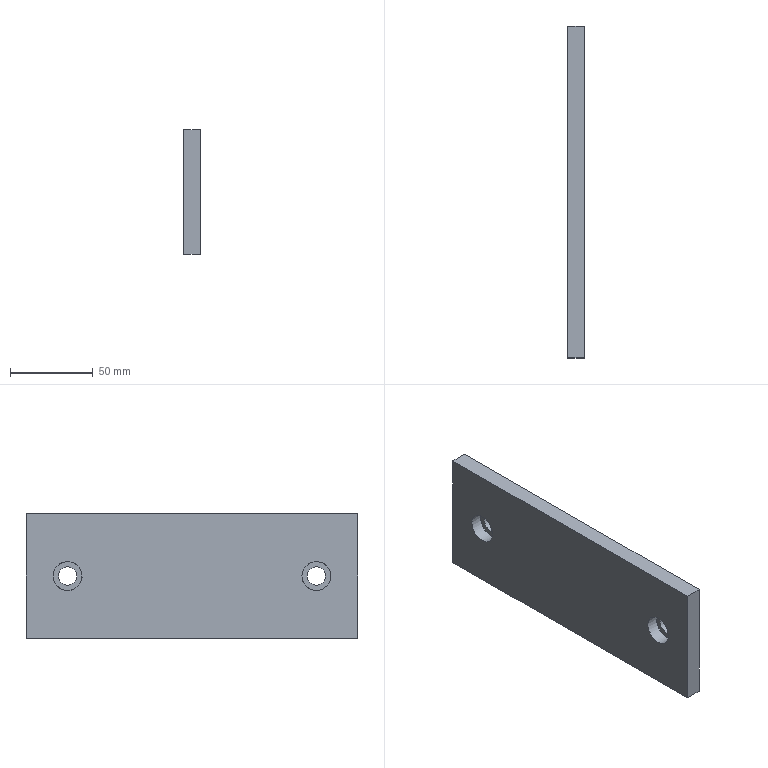Part | NX | features solid 2 | 1 solid | 12 faces | box 10 x 200 x 75 mm | volume 145975 mm3 | plane 8 | cylinder 4 | commonest cylinder face diameters 11 x2 17.5 x2
STEP:
#1=CARTESIAN_POINT('',(-680.,-535.,290.));
#2=VERTEX_POINT('',#1);
#3=CARTESIAN_POINT('',(-680.,-535.,215.));
#4=VERTEX_POINT('',#3);
#5=CARTESIAN_POINT('',(-680.,-535.,210.));
#6=DIRECTION('',(0.,0.,-1.));
#7=VECTOR('',#6,1000.);
#8=LINE('',#5,#7);
#9=EDGE_CURVE('',#2,#4,#8,.T.);
#10=ORIENTED_EDGE('',*,*,#9,.T.);
#11=CARTESIAN_POINT('',(-670.,-535.,215.));
#12=VERTEX_POINT('',#11);
#13=CARTESIAN_POINT('',(-670.,-535.,215.));
#14=DIRECTION('',(-1.,0.,0.));
#15=VECTOR('',#14,1000.);
#16=LINE('',#13,#15);
#17=EDGE_CURVE('',#12,#4,#16,.T.);
#18=ORIENTED_EDGE('',*,*,#17,.F.);
#19=CARTESIAN_POINT('',(-670.,-535.,290.));
#20=VERTEX_POINT('',#19);
#21=CARTESIAN_POINT('',(-670.,-535.,210.));
#22=DIRECTION('',(0.,0.,1.));
#23=VECTOR('',#22,1000.);
#24=LINE('',#21,#23);
#25=EDGE_CURVE('',#20,#12,#24,.F.);
#26=ORIENTED_EDGE('',*,*,#25,.F.);
#27=CARTESIAN_POINT('',(-670.,-535.,290.));
#28=DIRECTION('',(-1.,0.,0.));
#29=VECTOR('',#28,1000.);
#30=LINE('',#27,#29);
#31=EDGE_CURVE('',#20,#2,#30,.T.);
#32=ORIENTED_EDGE('',*,*,#31,.T.);
#33=EDGE_LOOP('',(#10,#18,#26,#32));
#34=FACE_BOUND('',#33,.T.);
#35=CARTESIAN_POINT('',(-670.,-535.,210.));
#36=DIRECTION('',(0.,1.,0.));
#37=DIRECTION('',(-1.,0.,0.));
#38=AXIS2_PLACEMENT_3D('',#35,#36,#37);
#39=PLANE('',#38);
#40=ADVANCED_FACE('',(#34),#39,.F.);
#41=CARTESIAN_POINT('',(-680.,-335.,290.));
#42=VERTEX_POINT('',#41);
#43=CARTESIAN_POINT('',(-680.,-485.,290.));
#44=DIRECTION('',(0.,-1.,0.));
#45=VECTOR('',#44,1000.);
#46=LINE('',#43,#45);
#47=EDGE_CURVE('',#42,#2,#46,.T.);
#48=ORIENTED_EDGE('',*,*,#47,.T.);
#49=ORIENTED_EDGE('',*,*,#31,.F.);
#50=CARTESIAN_POINT('',(-670.,-335.,290.));
#51=VERTEX_POINT('',#50);
#52=CARTESIAN_POINT('',(-670.,-485.,290.));
#53=DIRECTION('',(0.,-1.,0.));
#54=VECTOR('',#53,1000.);
#55=LINE('',#52,#54);
#56=EDGE_CURVE('',#51,#20,#55,.T.);
#57=ORIENTED_EDGE('',*,*,#56,.F.);
#58=CARTESIAN_POINT('',(-670.,-335.,290.));
#59=DIRECTION('',(-1.,0.,0.));
#60=VECTOR('',#59,1000.);
#61=LINE('',#58,#60);
#62=EDGE_CURVE('',#51,#42,#61,.T.);
#63=ORIENTED_EDGE('',*,*,#62,.T.);
#64=EDGE_LOOP('',(#48,#49,#57,#63));
#65=FACE_BOUND('',#64,.T.);
#66=CARTESIAN_POINT('',(-670.,-485.,290.));
#67=DIRECTION('',(0.,0.,-1.));
#68=DIRECTION('',(1.,0.,0.));
#69=AXIS2_PLACEMENT_3D('',#66,#67,#68);
#70=PLANE('',#69);
#71=ADVANCED_FACE('',(#65),#70,.F.);
#72=CARTESIAN_POINT('',(-680.,-335.,215.));
#73=VERTEX_POINT('',#72);
#74=CARTESIAN_POINT('',(-680.,-335.,268.));
#75=DIRECTION('',(0.,0.,1.));
#76=VECTOR('',#75,1000.);
#77=LINE('',#74,#76);
#78=EDGE_CURVE('',#73,#42,#77,.T.);
#79=ORIENTED_EDGE('',*,*,#78,.T.);
#80=ORIENTED_EDGE('',*,*,#62,.F.);
#81=CARTESIAN_POINT('',(-670.,-335.,215.));
#82=VERTEX_POINT('',#81);
#83=CARTESIAN_POINT('',(-670.,-335.,268.));
#84=DIRECTION('',(0.,0.,-1.));
#85=VECTOR('',#84,1000.);
#86=LINE('',#83,#85);
#87=EDGE_CURVE('',#82,#51,#86,.F.);
#88=ORIENTED_EDGE('',*,*,#87,.F.);
#89=CARTESIAN_POINT('',(-670.,-335.,215.));
#90=DIRECTION('',(-1.,0.,0.));
#91=VECTOR('',#90,1000.);
#92=LINE('',#89,#91);
#93=EDGE_CURVE('',#82,#73,#92,.T.);
#94=ORIENTED_EDGE('',*,*,#93,.T.);
#95=EDGE_LOOP('',(#79,#80,#88,#94));
#96=FACE_BOUND('',#95,.T.);
#97=CARTESIAN_POINT('',(-670.,-335.,268.));
#98=DIRECTION('',(0.,-1.,0.));
#99=DIRECTION('',(1.,0.,0.));
#100=AXIS2_PLACEMENT_3D('',#97,#98,#99);
#101=PLANE('',#100);
#102=ADVANCED_FACE('',(#96),#101,.F.);
#103=CARTESIAN_POINT('',(-680.,-335.,215.));
#104=DIRECTION('',(0.,1.,0.));
#105=VECTOR('',#104,1000.);
#106=LINE('',#103,#105);
#107=EDGE_CURVE('',#4,#73,#106,.T.);
#108=ORIENTED_EDGE('',*,*,#107,.T.);
#109=ORIENTED_EDGE('',*,*,#93,.F.);
#110=CARTESIAN_POINT('',(-670.,-485.,215.));
#111=DIRECTION('',(0.,1.,0.));
#112=VECTOR('',#111,1000.);
#113=LINE('',#110,#112);
#114=EDGE_CURVE('',#12,#82,#113,.T.);
#115=ORIENTED_EDGE('',*,*,#114,.F.);
#116=ORIENTED_EDGE('',*,*,#17,.T.);
#117=EDGE_LOOP('',(#108,#109,#115,#116));
#118=FACE_BOUND('',#117,.T.);
#119=CARTESIAN_POINT('',(-670.,-335.,215.));
#120=DIRECTION('',(0.,0.,1.));
#121=DIRECTION('',(0.,1.,0.));
#122=AXIS2_PLACEMENT_3D('',#119,#120,#121);
#123=PLANE('',#122);
#124=ADVANCED_FACE('',(#118),#123,.F.);
#125=CARTESIAN_POINT('',(-672.7,-501.25,252.5));
#126=VERTEX_POINT('',#125);
#127=CARTESIAN_POINT('',(-672.7,-510.,252.5));
#128=DIRECTION('',(-1.,0.,0.));
#129=DIRECTION('',(0.,1.,0.));
#130=AXIS2_PLACEMENT_3D('',#127,#128,#129);
#131=CIRCLE('',#130,8.75);
#132=EDGE_CURVE('',#126,#126,#131,.T.);
#133=ORIENTED_EDGE('',*,*,#132,.F.);
#134=EDGE_LOOP('',(#133));
#135=FACE_BOUND('',#134,.T.);
#136=CARTESIAN_POINT('',(-680.,-510.,243.75));
#137=VERTEX_POINT('',#136);
#138=CARTESIAN_POINT('',(-680.,-510.,252.5));
#139=DIRECTION('',(1.,0.,0.));
#140=DIRECTION('',(0.,0.,-1.));
#141=AXIS2_PLACEMENT_3D('',#138,#139,#140);
#142=CIRCLE('',#141,8.75);
#143=EDGE_CURVE('',#137,#137,#142,.F.);
#144=ORIENTED_EDGE('',*,*,#143,.T.);
#145=EDGE_LOOP('',(#144));
#146=FACE_BOUND('',#145,.T.);
#147=CARTESIAN_POINT('',(-690.,-510.,252.5));
#148=DIRECTION('',(1.,0.,0.));
#149=DIRECTION('',(0.,1.,0.));
#150=AXIS2_PLACEMENT_3D('',#147,#148,#149);
#151=CYLINDRICAL_SURFACE('',#150,8.75);
#152=ADVANCED_FACE('',(#135,#146),#151,.F.);
#153=CARTESIAN_POINT('',(-672.7,-351.25,252.5));
#154=VERTEX_POINT('',#153);
#155=CARTESIAN_POINT('',(-672.7,-360.,252.5));
#156=DIRECTION('',(-1.,0.,0.));
#157=DIRECTION('',(0.,1.,0.));
#158=AXIS2_PLACEMENT_3D('',#155,#156,#157);
#159=CIRCLE('',#158,8.75);
#160=EDGE_CURVE('',#154,#154,#159,.T.);
#161=ORIENTED_EDGE('',*,*,#160,.F.);
#162=EDGE_LOOP('',(#161));
#163=FACE_BOUND('',#162,.T.);
#164=CARTESIAN_POINT('',(-680.,-360.,243.75));
#165=VERTEX_POINT('',#164);
#166=CARTESIAN_POINT('',(-680.,-360.,252.5));
#167=DIRECTION('',(1.,0.,0.));
#168=DIRECTION('',(0.,0.,-1.));
#169=AXIS2_PLACEMENT_3D('',#166,#167,#168);
#170=CIRCLE('',#169,8.75);
#171=EDGE_CURVE('',#165,#165,#170,.F.);
#172=ORIENTED_EDGE('',*,*,#171,.T.);
#173=EDGE_LOOP('',(#172));
#174=FACE_BOUND('',#173,.T.);
#175=CARTESIAN_POINT('',(-690.,-360.,252.5));
#176=DIRECTION('',(1.,0.,0.));
#177=DIRECTION('',(0.,1.,0.));
#178=AXIS2_PLACEMENT_3D('',#175,#176,#177);
#179=CYLINDRICAL_SURFACE('',#178,8.75);
#180=ADVANCED_FACE('',(#163,#174),#179,.F.);
#181=CARTESIAN_POINT('',(-670.,-354.5,252.5));
#182=VERTEX_POINT('',#181);
#183=CARTESIAN_POINT('',(-670.,-360.,252.5));
#184=DIRECTION('',(-1.,0.,0.));
#185=DIRECTION('',(0.,1.,0.));
#186=AXIS2_PLACEMENT_3D('',#183,#184,#185);
#187=CIRCLE('',#186,5.5);
#188=EDGE_CURVE('',#182,#182,#187,.T.);
#189=ORIENTED_EDGE('',*,*,#188,.T.);
#190=EDGE_LOOP('',(#189));
#191=FACE_BOUND('',#190,.T.);
#192=CARTESIAN_POINT('',(-670.,-504.5,252.5));
#193=VERTEX_POINT('',#192);
#194=CARTESIAN_POINT('',(-670.,-510.,252.5));
#195=DIRECTION('',(-1.,0.,0.));
#196=DIRECTION('',(0.,1.,0.));
#197=AXIS2_PLACEMENT_3D('',#194,#195,#196);
#198=CIRCLE('',#197,5.5);
#199=EDGE_CURVE('',#193,#193,#198,.T.);
#200=ORIENTED_EDGE('',*,*,#199,.T.);
#201=EDGE_LOOP('',(#200));
#202=FACE_BOUND('',#201,.T.);
#203=ORIENTED_EDGE('',*,*,#87,.T.);
#204=ORIENTED_EDGE('',*,*,#56,.T.);
#205=ORIENTED_EDGE('',*,*,#25,.T.);
#206=ORIENTED_EDGE('',*,*,#114,.T.);
#207=EDGE_LOOP('',(#203,#204,#205,#206));
#208=FACE_BOUND('',#207,.T.);
#209=CARTESIAN_POINT('',(-670.,-485.,268.));
#210=DIRECTION('',(1.,0.,0.));
#211=DIRECTION('',(0.,1.,0.));
#212=AXIS2_PLACEMENT_3D('',#209,#210,#211);
#213=PLANE('',#212);
#214=ADVANCED_FACE('',(#191,#202,#208),#213,.T.);
#215=ORIENTED_EDGE('',*,*,#199,.F.);
#216=EDGE_LOOP('',(#215));
#217=FACE_BOUND('',#216,.T.);
#218=CARTESIAN_POINT('',(-672.7,-504.5,252.5));
#219=VERTEX_POINT('',#218);
#220=CARTESIAN_POINT('',(-672.7,-510.,252.5));
#221=DIRECTION('',(-1.,0.,0.));
#222=DIRECTION('',(0.,1.,0.));
#223=AXIS2_PLACEMENT_3D('',#220,#221,#222);
#224=CIRCLE('',#223,5.5);
#225=EDGE_CURVE('',#219,#219,#224,.T.);
#226=ORIENTED_EDGE('',*,*,#225,.T.);
#227=EDGE_LOOP('',(#226));
#228=FACE_BOUND('',#227,.T.);
#229=CARTESIAN_POINT('',(-640.,-510.,252.5));
#230=DIRECTION('',(1.,0.,0.));
#231=DIRECTION('',(0.,1.,0.));
#232=AXIS2_PLACEMENT_3D('',#229,#230,#231);
#233=CYLINDRICAL_SURFACE('',#232,5.5);
#234=ADVANCED_FACE('',(#217,#228),#233,.F.);
#235=ORIENTED_EDGE('',*,*,#225,.F.);
#236=EDGE_LOOP('',(#235));
#237=FACE_BOUND('',#236,.T.);
#238=ORIENTED_EDGE('',*,*,#132,.T.);
#239=EDGE_LOOP('',(#238));
#240=FACE_BOUND('',#239,.T.);
#241=CARTESIAN_POINT('',(-672.7,-510.,252.5));
#242=DIRECTION('',(1.,0.,0.));
#243=DIRECTION('',(0.,1.,0.));
#244=AXIS2_PLACEMENT_3D('',#241,#242,#243);
#245=PLANE('',#244);
#246=ADVANCED_FACE('',(#237,#240),#245,.F.);
#247=ORIENTED_EDGE('',*,*,#188,.F.);
#248=EDGE_LOOP('',(#247));
#249=FACE_BOUND('',#248,.T.);
#250=CARTESIAN_POINT('',(-672.7,-354.5,252.5));
#251=VERTEX_POINT('',#250);
#252=CARTESIAN_POINT('',(-672.7,-360.,252.5));
#253=DIRECTION('',(-1.,0.,0.));
#254=DIRECTION('',(0.,1.,0.));
#255=AXIS2_PLACEMENT_3D('',#252,#253,#254);
#256=CIRCLE('',#255,5.5);
#257=EDGE_CURVE('',#251,#251,#256,.T.);
#258=ORIENTED_EDGE('',*,*,#257,.T.);
#259=EDGE_LOOP('',(#258));
#260=FACE_BOUND('',#259,.T.);
#261=CARTESIAN_POINT('',(-640.,-360.,252.5));
#262=DIRECTION('',(1.,0.,0.));
#263=DIRECTION('',(0.,1.,0.));
#264=AXIS2_PLACEMENT_3D('',#261,#262,#263);
#265=CYLINDRICAL_SURFACE('',#264,5.5);
#266=ADVANCED_FACE('',(#249,#260),#265,.F.);
#267=ORIENTED_EDGE('',*,*,#257,.F.);
#268=EDGE_LOOP('',(#267));
#269=FACE_BOUND('',#268,.T.);
#270=ORIENTED_EDGE('',*,*,#160,.T.);
#271=EDGE_LOOP('',(#270));
#272=FACE_BOUND('',#271,.T.);
#273=CARTESIAN_POINT('',(-672.7,-360.,252.5));
#274=DIRECTION('',(1.,0.,0.));
#275=DIRECTION('',(0.,1.,0.));
#276=AXIS2_PLACEMENT_3D('',#273,#274,#275);
#277=PLANE('',#276);
#278=ADVANCED_FACE('',(#269,#272),#277,.F.);
#279=ORIENTED_EDGE('',*,*,#143,.F.);
#280=EDGE_LOOP('',(#279));
#281=FACE_BOUND('',#280,.T.);
#282=ORIENTED_EDGE('',*,*,#171,.F.);
#283=EDGE_LOOP('',(#282));
#284=FACE_BOUND('',#283,.T.);
#285=ORIENTED_EDGE('',*,*,#47,.F.);
#286=ORIENTED_EDGE('',*,*,#78,.F.);
#287=ORIENTED_EDGE('',*,*,#107,.F.);
#288=ORIENTED_EDGE('',*,*,#9,.F.);
#289=EDGE_LOOP('',(#285,#286,#287,#288));
#290=FACE_BOUND('',#289,.T.);
#291=CARTESIAN_POINT('',(-680.,-410.,239.));
#292=DIRECTION('',(-1.,0.,0.));
#293=DIRECTION('',(0.,0.,-1.));
#294=AXIS2_PLACEMENT_3D('',#291,#292,#293);
#295=PLANE('',#294);
#296=ADVANCED_FACE('',(#281,#284,#290),#295,.T.);
#297=CLOSED_SHELL('',(#40,#71,#102,#124,#152,#180,#214,#234,#246,#266,#278,#296));
#298=MANIFOLD_SOLID_BREP('',#297);
#299=(LENGTH_UNIT()NAMED_UNIT(*)SI_UNIT(.MILLI.,.METRE.));
#300=UNCERTAINTY_MEASURE_WITH_UNIT(LENGTH_MEASURE(0.00001),#299,'','');
#301=(NAMED_UNIT(*)PLANE_ANGLE_UNIT()SI_UNIT($,.RADIAN.));
#302=(NAMED_UNIT(*)SI_UNIT($,.STERADIAN.)SOLID_ANGLE_UNIT());
#303=(GEOMETRIC_REPRESENTATION_CONTEXT(3)GLOBAL_UNCERTAINTY_ASSIGNED_CONTEXT((#300))GLOBAL_UNIT_ASSIGNED_CONTEXT((#299,#301,#302))REPRESENTATION_CONTEXT('',''));
#304=ADVANCED_BREP_SHAPE_REPRESENTATION('',(#298),#303);